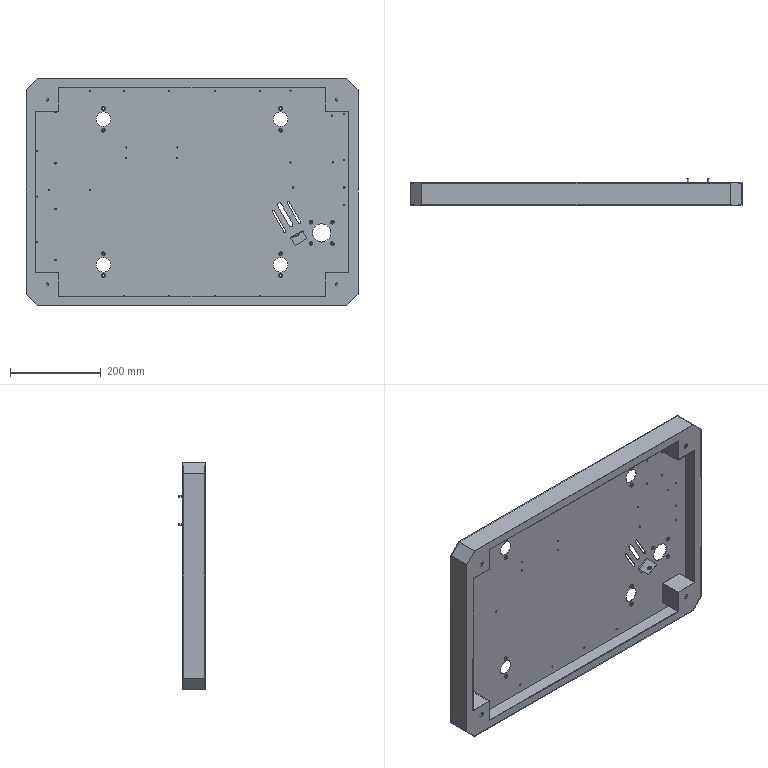Part | SolidWorks | features BaseBody 1 | 1 solid | 264 faces | box 730 x 58.5 x 500 mm | volume 825943 mm3 | cylinder 173 | plane 83 | cone 8 | commonest cylinder face diameters 2.5 x56 3.3 x30 4.2 x26 8.7 x18 5 x14 7.9 x8